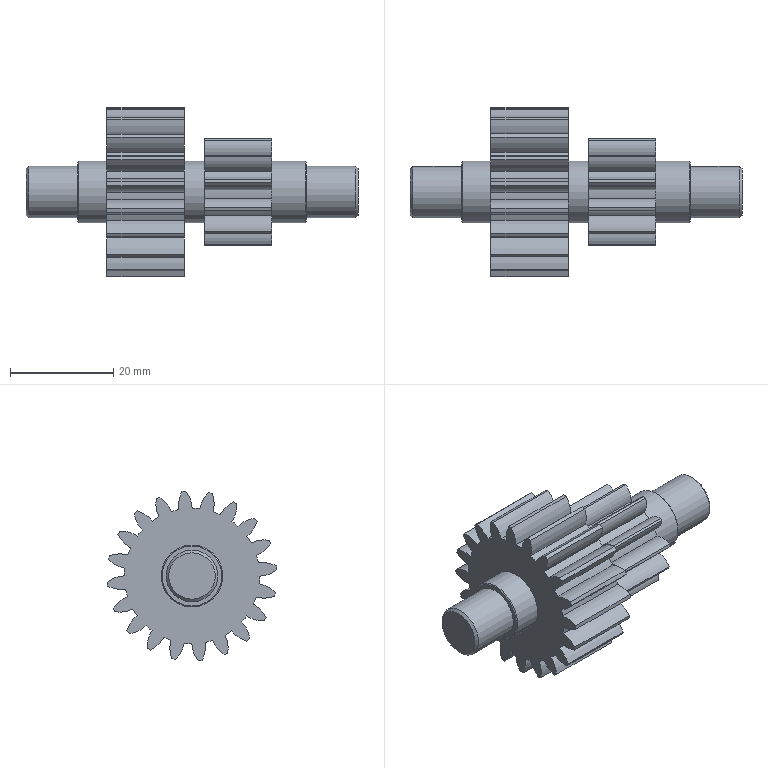Part | NX | features BREP 1 | 1 solid | 145 faces | box 64.4 x 32.912 x 32.912 mm | volume 16745 mm3 | cylinder 133 | plane 8 | cone 4 | commonest cylinder face diameters 12 x43 7.2 x24 26.248 x20 32.998 x20 14.248 x12 21.05 x12